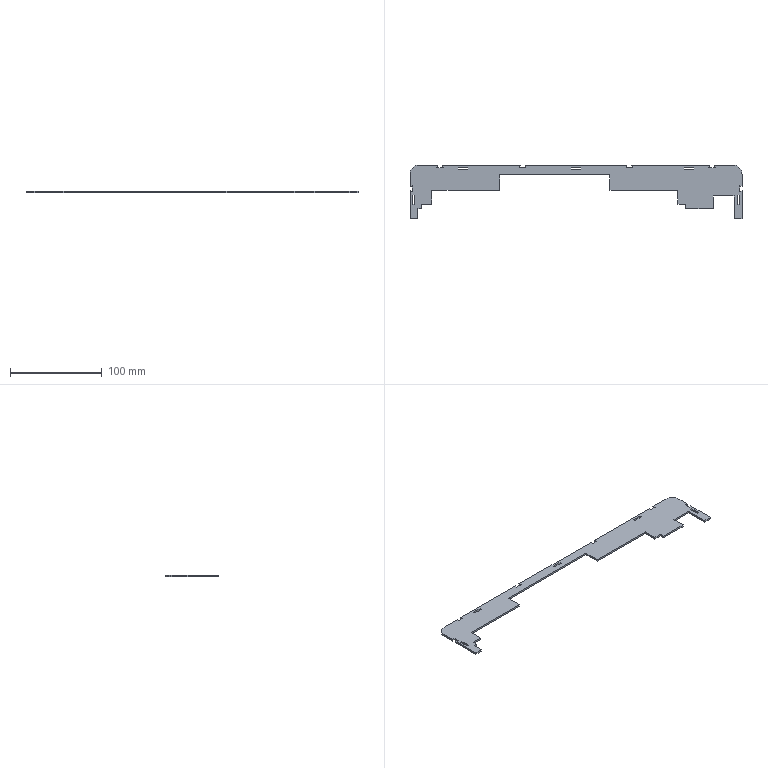Part | STEP file | xzz-005-1 | 1 solid | 70 faces | box 361.4 x 58.7 x 2 mm | volume 18757 mm3 | plane 68 | cylinder 2 | commonest cylinder face diameters 20 x2